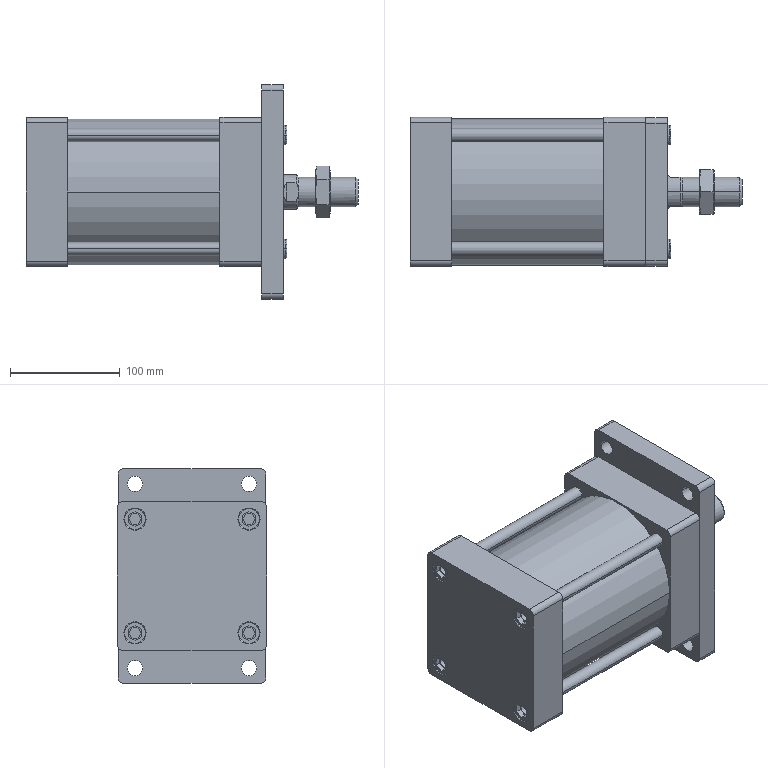Part | STEP file | SC125X100SFA_000_ | 4 solids | 352 faces | box 303 x 136 x 196 mm | volume 2823213 mm3 | plane 169 | cylinder 116 | cone 57 | torus 10 | commonest cylinder face diameters 10.106 x16 12 x16 19.2 x16 10 x12 14 x8 18 x8